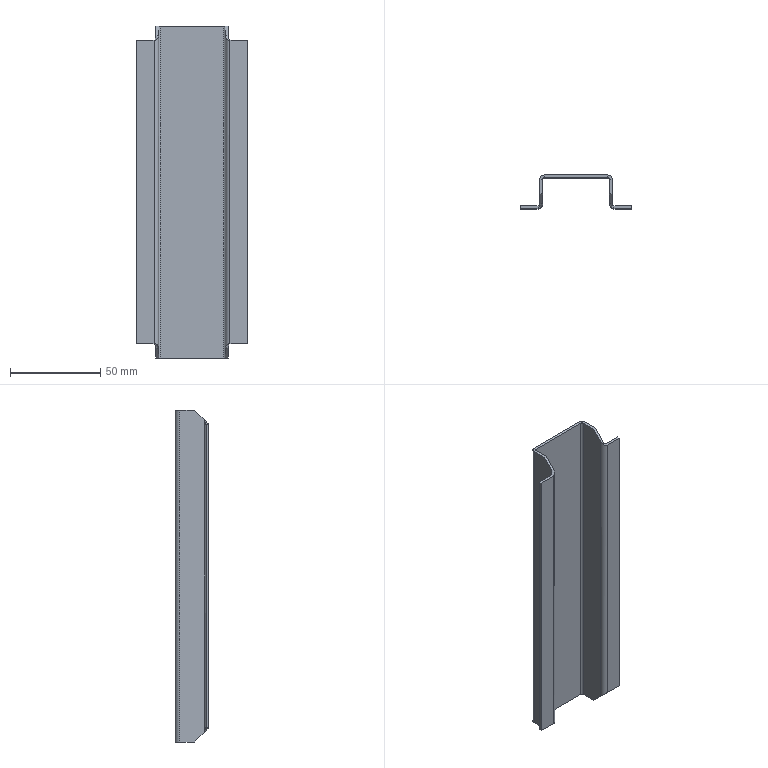Part | SolidWorks | features FlatPattern 1, ICE 1, SMBaseFlange 1, SheetMetal 1 | 1 solid | 42 faces | box 61 x 18.5 x 183.5 mm | volume 24658 mm3 | plane 30 | cylinder 8 | spline 4 | commonest cylinder face diameters 2 x4 5 x4
STEP:
#1=CARTESIAN_POINT('',(22.477,26.708,8.));
#2=VERTEX_POINT('',#1);
#3=CARTESIAN_POINT('',(12.977,26.708,8.));
#4=VERTEX_POINT('',#3);
#5=CARTESIAN_POINT('',(168.477,26.708,8.));
#6=DIRECTION('',(-1.,0.,0.));
#7=VECTOR('',#6,1000.);
#8=LINE('',#5,#7);
#9=EDGE_CURVE('',#2,#4,#8,.T.);
#10=ORIENTED_EDGE('',*,*,#9,.F.);
#11=CARTESIAN_POINT('',(22.477,26.708,175.5));
#12=VERTEX_POINT('',#11);
#13=CARTESIAN_POINT('',(22.477,26.708,183.5));
#14=DIRECTION('',(0.,0.,-1.));
#15=VECTOR('',#14,1000.);
#16=LINE('',#13,#15);
#17=EDGE_CURVE('',#12,#2,#16,.T.);
#18=ORIENTED_EDGE('',*,*,#17,.F.);
#19=CARTESIAN_POINT('',(12.977,26.708,175.5));
#20=VERTEX_POINT('',#19);
#21=CARTESIAN_POINT('',(168.477,26.708,175.5));
#22=DIRECTION('',(-1.,0.,0.));
#23=VECTOR('',#22,1000.);
#24=LINE('',#21,#23);
#25=EDGE_CURVE('',#12,#20,#24,.T.);
#26=ORIENTED_EDGE('',*,*,#25,.T.);
#27=CARTESIAN_POINT('',(12.977,26.708,183.5));
#28=DIRECTION('',(0.,0.,-1.));
#29=VECTOR('',#28,1000.);
#30=LINE('',#27,#29);
#31=EDGE_CURVE('',#20,#4,#30,.T.);
#32=ORIENTED_EDGE('',*,*,#31,.T.);
#33=EDGE_LOOP('',(#10,#18,#26,#32));
#34=FACE_OUTER_BOUND('',#33,.T.);
#35=CARTESIAN_POINT('',(11.977,26.708,183.5));
#36=DIRECTION('',(0.,1.,0.));
#37=DIRECTION('',(-1.,0.,0.));
#38=AXIS2_PLACEMENT_3D('',#35,#36,#37);
#39=PLANE('',#38);
#40=ADVANCED_FACE('',(#34),#39,.F.);
#41=ORIENTED_EDGE('',*,*,#17,.T.);
#42=CARTESIAN_POINT('',(22.477,28.208,8.));
#43=VERTEX_POINT('',#42);
#44=CARTESIAN_POINT('',(22.477,26.708,8.));
#45=DIRECTION('',(0.,1.,0.));
#46=VECTOR('',#45,1000.);
#47=LINE('',#44,#46);
#48=EDGE_CURVE('',#2,#43,#47,.T.);
#49=ORIENTED_EDGE('',*,*,#48,.T.);
#50=CARTESIAN_POINT('',(22.477,28.208,175.5));
#51=VERTEX_POINT('',#50);
#52=CARTESIAN_POINT('',(22.477,28.208,183.5));
#53=DIRECTION('',(0.,0.,-1.));
#54=VECTOR('',#53,1000.);
#55=LINE('',#52,#54);
#56=EDGE_CURVE('',#51,#43,#55,.T.);
#57=ORIENTED_EDGE('',*,*,#56,.F.);
#58=CARTESIAN_POINT('',(22.477,26.708,175.5));
#59=DIRECTION('',(0.,1.,0.));
#60=VECTOR('',#59,1000.);
#61=LINE('',#58,#60);
#62=EDGE_CURVE('',#12,#51,#61,.T.);
#63=ORIENTED_EDGE('',*,*,#62,.F.);
#64=EDGE_LOOP('',(#41,#49,#57,#63));
#65=FACE_OUTER_BOUND('',#64,.T.);
#66=CARTESIAN_POINT('',(22.477,28.208,183.5));
#67=DIRECTION('',(1.,0.,0.));
#68=DIRECTION('',(0.,0.,-1.));
#69=AXIS2_PLACEMENT_3D('',#66,#67,#68);
#70=PLANE('',#69);
#71=ADVANCED_FACE('',(#65),#70,.T.);
#72=ORIENTED_EDGE('',*,*,#56,.T.);
#73=CARTESIAN_POINT('',(12.977,28.208,8.));
#74=VERTEX_POINT('',#73);
#75=CARTESIAN_POINT('',(11.977,28.208,8.));
#76=DIRECTION('',(-1.,0.,0.));
#77=VECTOR('',#76,1000.);
#78=LINE('',#75,#77);
#79=EDGE_CURVE('',#43,#74,#78,.T.);
#80=ORIENTED_EDGE('',*,*,#79,.T.);
#81=CARTESIAN_POINT('',(12.977,28.208,175.5));
#82=VERTEX_POINT('',#81);
#83=CARTESIAN_POINT('',(12.977,28.208,183.5));
#84=DIRECTION('',(0.,0.,-1.));
#85=VECTOR('',#84,1000.);
#86=LINE('',#83,#85);
#87=EDGE_CURVE('',#82,#74,#86,.T.);
#88=ORIENTED_EDGE('',*,*,#87,.F.);
#89=CARTESIAN_POINT('',(11.977,28.208,175.5));
#90=DIRECTION('',(-1.,0.,0.));
#91=VECTOR('',#90,1000.);
#92=LINE('',#89,#91);
#93=EDGE_CURVE('',#51,#82,#92,.T.);
#94=ORIENTED_EDGE('',*,*,#93,.F.);
#95=EDGE_LOOP('',(#72,#80,#88,#94));
#96=FACE_OUTER_BOUND('',#95,.T.);
#97=CARTESIAN_POINT('',(11.977,28.208,183.5));
#98=DIRECTION('',(0.,1.,0.));
#99=DIRECTION('',(-1.,0.,0.));
#100=AXIS2_PLACEMENT_3D('',#97,#98,#99);
#101=PLANE('',#100);
#102=ADVANCED_FACE('',(#96),#101,.T.);
#103=ORIENTED_EDGE('',*,*,#87,.T.);
#104=CARTESIAN_POINT('',(11.977,29.208,5.5));
#105=VERTEX_POINT('',#104);
#106=CARTESIAN_POINT('',(11.977,29.208,5.5));
#107=CARTESIAN_POINT('',(11.977,28.623,6.964));
#108=CARTESIAN_POINT('',(12.391,28.208,8.));
#109=CARTESIAN_POINT('',(12.977,28.208,8.));
#110=(BOUNDED_CURVE()B_SPLINE_CURVE(3,(#106,#107,#108,#109),.UNSPECIFIED.,.F.,.T.)B_SPLINE_CURVE_WITH_KNOTS((4,4),(1.571,3.142),.UNSPECIFIED.)CURVE()GEOMETRIC_REPRESENTATION_ITEM()RATIONAL_B_SPLINE_CURVE((1.,0.8047,0.8047,1.))REPRESENTATION_ITEM(''));
#111=EDGE_CURVE('',#105,#74,#110,.T.);
#112=ORIENTED_EDGE('',*,*,#111,.F.);
#113=CARTESIAN_POINT('',(11.977,29.208,178.));
#114=VERTEX_POINT('',#113);
#115=CARTESIAN_POINT('',(11.977,29.208,183.5));
#116=DIRECTION('',(0.,0.,-1.));
#117=VECTOR('',#116,1000.);
#118=LINE('',#115,#117);
#119=EDGE_CURVE('',#114,#105,#118,.T.);
#120=ORIENTED_EDGE('',*,*,#119,.F.);
#121=CARTESIAN_POINT('',(12.977,28.208,175.5));
#122=CARTESIAN_POINT('',(12.391,28.208,175.5));
#123=CARTESIAN_POINT('',(11.977,28.623,176.536));
#124=CARTESIAN_POINT('',(11.977,29.208,178.));
#125=(BOUNDED_CURVE()B_SPLINE_CURVE(3,(#121,#122,#123,#124),.UNSPECIFIED.,.F.,.T.)B_SPLINE_CURVE_WITH_KNOTS((4,4),(0.,1.571),.UNSPECIFIED.)CURVE()GEOMETRIC_REPRESENTATION_ITEM()RATIONAL_B_SPLINE_CURVE((1.,0.8047,0.8047,1.))REPRESENTATION_ITEM(''));
#126=EDGE_CURVE('',#82,#114,#125,.T.);
#127=ORIENTED_EDGE('',*,*,#126,.F.);
#128=EDGE_LOOP('',(#103,#112,#120,#127));
#129=FACE_OUTER_BOUND('',#128,.T.);
#130=CARTESIAN_POINT('',(12.977,29.208,183.5));
#131=DIRECTION('',(0.,0.,-1.));
#132=DIRECTION('',(-1.,0.,0.));
#133=AXIS2_PLACEMENT_3D('',#130,#131,#132);
#134=CYLINDRICAL_SURFACE('',#133,1.);
#135=ADVANCED_FACE('',(#129),#134,.F.);
#136=ORIENTED_EDGE('',*,*,#119,.T.);
#137=CARTESIAN_POINT('',(11.977,34.708,0.));
#138=VERTEX_POINT('',#137);
#139=CARTESIAN_POINT('',(11.977,-51.792,86.5));
#140=DIRECTION('',(0.,-0.7071,0.7071));
#141=VECTOR('',#140,1000.);
#142=LINE('',#139,#141);
#143=EDGE_CURVE('',#138,#105,#142,.T.);
#144=ORIENTED_EDGE('',*,*,#143,.F.);
#145=CARTESIAN_POINT('',(11.977,42.708,0.));
#146=VERTEX_POINT('',#145);
#147=CARTESIAN_POINT('',(11.977,45.208,0.));
#148=DIRECTION('',(0.,-1.,0.));
#149=VECTOR('',#148,1000.);
#150=LINE('',#147,#149);
#151=EDGE_CURVE('',#146,#138,#150,.T.);
#152=ORIENTED_EDGE('',*,*,#151,.F.);
#153=CARTESIAN_POINT('',(11.977,42.708,183.5));
#154=VERTEX_POINT('',#153);
#155=CARTESIAN_POINT('',(11.977,42.708,183.5));
#156=DIRECTION('',(0.,0.,-1.));
#157=VECTOR('',#156,1000.);
#158=LINE('',#155,#157);
#159=EDGE_CURVE('',#154,#146,#158,.T.);
#160=ORIENTED_EDGE('',*,*,#159,.F.);
#161=CARTESIAN_POINT('',(11.977,34.708,183.5));
#162=VERTEX_POINT('',#161);
#163=CARTESIAN_POINT('',(11.977,45.208,183.5));
#164=DIRECTION('',(0.,-1.,0.));
#165=VECTOR('',#164,1000.);
#166=LINE('',#163,#165);
#167=EDGE_CURVE('',#154,#162,#166,.T.);
#168=ORIENTED_EDGE('',*,*,#167,.T.);
#169=CARTESIAN_POINT('',(11.977,39.958,188.75));
#170=DIRECTION('',(0.,0.7071,0.7071));
#171=VECTOR('',#170,1000.);
#172=LINE('',#169,#171);
#173=EDGE_CURVE('',#114,#162,#172,.T.);
#174=ORIENTED_EDGE('',*,*,#173,.F.);
#175=EDGE_LOOP('',(#136,#144,#152,#160,#168,#174));
#176=FACE_OUTER_BOUND('',#175,.T.);
#177=CARTESIAN_POINT('',(11.977,45.208,183.5));
#178=DIRECTION('',(1.,0.,0.));
#179=DIRECTION('',(0.,1.,0.));
#180=AXIS2_PLACEMENT_3D('',#177,#178,#179);
#181=PLANE('',#180);
#182=ADVANCED_FACE('',(#176),#181,.T.);
#183=CARTESIAN_POINT('',(10.477,34.708,0.));
#184=VERTEX_POINT('',#183);
#185=CARTESIAN_POINT('',(10.477,29.208,5.5));
#186=VERTEX_POINT('',#185);
#187=CARTESIAN_POINT('',(10.477,-51.792,86.5));
#188=DIRECTION('',(0.,-0.7071,0.7071));
#189=VECTOR('',#188,1000.);
#190=LINE('',#187,#189);
#191=EDGE_CURVE('',#184,#186,#190,.T.);
#192=ORIENTED_EDGE('',*,*,#191,.T.);
#193=CARTESIAN_POINT('',(10.477,29.208,178.));
#194=VERTEX_POINT('',#193);
#195=CARTESIAN_POINT('',(10.477,29.208,183.5));
#196=DIRECTION('',(0.,0.,-1.));
#197=VECTOR('',#196,1000.);
#198=LINE('',#195,#197);
#199=EDGE_CURVE('',#194,#186,#198,.T.);
#200=ORIENTED_EDGE('',*,*,#199,.F.);
#201=CARTESIAN_POINT('',(10.477,34.708,183.5));
#202=VERTEX_POINT('',#201);
#203=CARTESIAN_POINT('',(10.477,39.958,188.75));
#204=DIRECTION('',(0.,0.7071,0.7071));
#205=VECTOR('',#204,1000.);
#206=LINE('',#203,#205);
#207=EDGE_CURVE('',#194,#202,#206,.T.);
#208=ORIENTED_EDGE('',*,*,#207,.T.);
#209=CARTESIAN_POINT('',(10.477,42.708,183.5));
#210=VERTEX_POINT('',#209);
#211=CARTESIAN_POINT('',(10.477,45.208,183.5));
#212=DIRECTION('',(0.,-1.,0.));
#213=VECTOR('',#212,1000.);
#214=LINE('',#211,#213);
#215=EDGE_CURVE('',#210,#202,#214,.T.);
#216=ORIENTED_EDGE('',*,*,#215,.F.);
#217=CARTESIAN_POINT('',(10.477,42.708,0.));
#218=VERTEX_POINT('',#217);
#219=CARTESIAN_POINT('',(10.477,42.708,183.5));
#220=DIRECTION('',(0.,0.,-1.));
#221=VECTOR('',#220,1000.);
#222=LINE('',#219,#221);
#223=EDGE_CURVE('',#210,#218,#222,.T.);
#224=ORIENTED_EDGE('',*,*,#223,.T.);
#225=CARTESIAN_POINT('',(10.477,45.208,0.));
#226=DIRECTION('',(0.,-1.,0.));
#227=VECTOR('',#226,1000.);
#228=LINE('',#225,#227);
#229=EDGE_CURVE('',#218,#184,#228,.T.);
#230=ORIENTED_EDGE('',*,*,#229,.T.);
#231=EDGE_LOOP('',(#192,#200,#208,#216,#224,#230));
#232=FACE_OUTER_BOUND('',#231,.T.);
#233=CARTESIAN_POINT('',(10.477,45.208,183.5));
#234=DIRECTION('',(1.,0.,0.));
#235=DIRECTION('',(0.,1.,0.));
#236=AXIS2_PLACEMENT_3D('',#233,#234,#235);
#237=PLANE('',#236);
#238=ADVANCED_FACE('',(#232),#237,.F.);
#239=CARTESIAN_POINT('',(10.477,29.208,5.5));
#240=CARTESIAN_POINT('',(10.477,27.744,6.964));
#241=CARTESIAN_POINT('',(11.512,26.708,8.));
#242=CARTESIAN_POINT('',(12.977,26.708,8.));
#243=(BOUNDED_CURVE()B_SPLINE_CURVE(3,(#239,#240,#241,#242),.UNSPECIFIED.,.F.,.T.)B_SPLINE_CURVE_WITH_KNOTS((4,4),(1.571,3.142),.UNSPECIFIED.)CURVE()GEOMETRIC_REPRESENTATION_ITEM()RATIONAL_B_SPLINE_CURVE((1.,0.8047,0.8047,1.))REPRESENTATION_ITEM(''));
#244=EDGE_CURVE('',#186,#4,#243,.T.);
#245=ORIENTED_EDGE('',*,*,#244,.T.);
#246=ORIENTED_EDGE('',*,*,#31,.F.);
#247=CARTESIAN_POINT('',(12.977,26.708,175.5));
#248=CARTESIAN_POINT('',(11.512,26.708,175.5));
#249=CARTESIAN_POINT('',(10.477,27.744,176.536));
#250=CARTESIAN_POINT('',(10.477,29.208,178.));
#251=(BOUNDED_CURVE()B_SPLINE_CURVE(3,(#247,#248,#249,#250),.UNSPECIFIED.,.F.,.T.)B_SPLINE_CURVE_WITH_KNOTS((4,4),(0.,1.571),.UNSPECIFIED.)CURVE()GEOMETRIC_REPRESENTATION_ITEM()RATIONAL_B_SPLINE_CURVE((1.,0.8047,0.8047,1.))REPRESENTATION_ITEM(''));
#252=EDGE_CURVE('',#20,#194,#251,.T.);
#253=ORIENTED_EDGE('',*,*,#252,.T.);
#254=ORIENTED_EDGE('',*,*,#199,.T.);
#255=EDGE_LOOP('',(#245,#246,#253,#254));
#256=FACE_OUTER_BOUND('',#255,.T.);
#257=CARTESIAN_POINT('',(12.977,29.208,183.5));
#258=DIRECTION('',(0.,0.,-1.));
#259=DIRECTION('',(-1.,0.,0.));
#260=AXIS2_PLACEMENT_3D('',#257,#258,#259);
#261=CYLINDRICAL_SURFACE('',#260,2.5);
#262=ADVANCED_FACE('',(#256),#261,.T.);
#263=CARTESIAN_POINT('',(-28.023,34.708,0.));
#264=VERTEX_POINT('',#263);
#265=CARTESIAN_POINT('',(-28.023,42.708,0.));
#266=VERTEX_POINT('',#265);
#267=CARTESIAN_POINT('',(-28.023,28.208,0.));
#268=DIRECTION('',(0.,1.,0.));
#269=VECTOR('',#268,1000.);
#270=LINE('',#267,#269);
#271=EDGE_CURVE('',#264,#266,#270,.T.);
#272=ORIENTED_EDGE('',*,*,#271,.F.);
#273=CARTESIAN_POINT('',(-28.023,29.208,5.5));
#274=VERTEX_POINT('',#273);
#275=CARTESIAN_POINT('',(-28.023,-60.292,95.));
#276=DIRECTION('',(0.,0.7071,-0.7071));
#277=VECTOR('',#276,1000.);
#278=LINE('',#275,#277);
#279=EDGE_CURVE('',#274,#264,#278,.T.);
#280=ORIENTED_EDGE('',*,*,#279,.F.);
#281=CARTESIAN_POINT('',(-28.023,29.208,178.));
#282=VERTEX_POINT('',#281);
#283=CARTESIAN_POINT('',(-28.023,29.208,183.5));
#284=DIRECTION('',(0.,0.,-1.));
#285=VECTOR('',#284,1000.);
#286=LINE('',#283,#285);
#287=EDGE_CURVE('',#282,#274,#286,.T.);
#288=ORIENTED_EDGE('',*,*,#287,.F.);
#289=CARTESIAN_POINT('',(-28.023,34.708,183.5));
#290=VERTEX_POINT('',#289);
#291=CARTESIAN_POINT('',(-28.023,31.458,180.25));
#292=DIRECTION('',(0.,-0.7071,-0.7071));
#293=VECTOR('',#292,1000.);
#294=LINE('',#291,#293);
#295=EDGE_CURVE('',#290,#282,#294,.T.);
#296=ORIENTED_EDGE('',*,*,#295,.F.);
#297=CARTESIAN_POINT('',(-28.023,42.708,183.5));
#298=VERTEX_POINT('',#297);
#299=CARTESIAN_POINT('',(-28.023,28.208,183.5));
#300=DIRECTION('',(0.,1.,0.));
#301=VECTOR('',#300,1000.);
#302=LINE('',#299,#301);
#303=EDGE_CURVE('',#290,#298,#302,.T.);
#304=ORIENTED_EDGE('',*,*,#303,.T.);
#305=CARTESIAN_POINT('',(-28.023,42.708,183.5));
#306=DIRECTION('',(0.,0.,-1.));
#307=VECTOR('',#306,1000.);
#308=LINE('',#305,#307);
#309=EDGE_CURVE('',#298,#266,#308,.T.);
#310=ORIENTED_EDGE('',*,*,#309,.T.);
#311=EDGE_LOOP('',(#272,#280,#288,#296,#304,#310));
#312=FACE_OUTER_BOUND('',#311,.T.);
#313=CARTESIAN_POINT('',(-28.023,28.208,183.5));
#314=DIRECTION('',(-1.,0.,0.));
#315=DIRECTION('',(0.,0.,1.));
#316=AXIS2_PLACEMENT_3D('',#313,#314,#315);
#317=PLANE('',#316);
#318=ADVANCED_FACE('',(#312),#317,.T.);
#319=ORIENTED_EDGE('',*,*,#287,.T.);
#320=CARTESIAN_POINT('',(-29.023,28.208,8.));
#321=VERTEX_POINT('',#320);
#322=CARTESIAN_POINT('',(-29.023,28.208,8.));
#323=CARTESIAN_POINT('',(-28.437,28.208,8.));
#324=CARTESIAN_POINT('',(-28.023,28.623,6.964));
#325=CARTESIAN_POINT('',(-28.023,29.208,5.5));
#326=(BOUNDED_CURVE()B_SPLINE_CURVE(3,(#322,#323,#324,#325),.UNSPECIFIED.,.F.,.T.)B_SPLINE_CURVE_WITH_KNOTS((4,4),(3.142,4.712),.UNSPECIFIED.)CURVE()GEOMETRIC_REPRESENTATION_ITEM()RATIONAL_B_SPLINE_CURVE((1.,0.8047,0.8047,1.))REPRESENTATION_ITEM(''));
#327=EDGE_CURVE('',#321,#274,#326,.T.);
#328=ORIENTED_EDGE('',*,*,#327,.F.);
#329=CARTESIAN_POINT('',(-29.023,28.208,175.5));
#330=VERTEX_POINT('',#329);
#331=CARTESIAN_POINT('',(-29.023,28.208,183.5));
#332=DIRECTION('',(0.,0.,-1.));
#333=VECTOR('',#332,1000.);
#334=LINE('',#331,#333);
#335=EDGE_CURVE('',#330,#321,#334,.T.);
#336=ORIENTED_EDGE('',*,*,#335,.F.);
#337=CARTESIAN_POINT('',(-28.023,29.208,178.));
#338=CARTESIAN_POINT('',(-28.023,28.623,176.536));
#339=CARTESIAN_POINT('',(-28.437,28.208,175.5));
#340=CARTESIAN_POINT('',(-29.023,28.208,175.5));
#341=(BOUNDED_CURVE()B_SPLINE_CURVE(3,(#337,#338,#339,#340),.UNSPECIFIED.,.F.,.T.)B_SPLINE_CURVE_WITH_KNOTS((4,4),(4.712,6.283),.UNSPECIFIED.)CURVE()GEOMETRIC_REPRESENTATION_ITEM()RATIONAL_B_SPLINE_CURVE((1.,0.8047,0.8047,1.))REPRESENTATION_ITEM(''));
#342=EDGE_CURVE('',#282,#330,#341,.T.);
#343=ORIENTED_EDGE('',*,*,#342,.F.);
#344=EDGE_LOOP('',(#319,#328,#336,#343));
#345=FACE_OUTER_BOUND('',#344,.T.);
#346=CARTESIAN_POINT('',(-29.023,29.208,183.5));
#347=DIRECTION('',(0.,0.,-1.));
#348=DIRECTION('',(-1.,0.,0.));
#349=AXIS2_PLACEMENT_3D('',#346,#347,#348);
#350=CYLINDRICAL_SURFACE('',#349,1.);
#351=ADVANCED_FACE('',(#345),#350,.F.);
#352=ORIENTED_EDGE('',*,*,#335,.T.);
#353=CARTESIAN_POINT('',(-38.523,28.208,8.));
#354=VERTEX_POINT('',#353);
#355=CARTESIAN_POINT('',(-38.523,28.208,8.));
#356=DIRECTION('',(-1.,0.,0.));
#357=VECTOR('',#356,1000.);
#358=LINE('',#355,#357);
#359=EDGE_CURVE('',#321,#354,#358,.T.);
#360=ORIENTED_EDGE('',*,*,#359,.T.);
#361=CARTESIAN_POINT('',(-38.523,28.208,175.5));
#362=VERTEX_POINT('',#361);
#363=CARTESIAN_POINT('',(-38.523,28.208,183.5));
#364=DIRECTION('',(0.,0.,-1.));
#365=VECTOR('',#364,1000.);
#366=LINE('',#363,#365);
#367=EDGE_CURVE('',#362,#354,#366,.T.);
#368=ORIENTED_EDGE('',*,*,#367,.F.);
#369=CARTESIAN_POINT('',(-38.523,28.208,175.5));
#370=DIRECTION('',(-1.,0.,0.));
#371=VECTOR('',#370,1000.);
#372=LINE('',#369,#371);
#373=EDGE_CURVE('',#330,#362,#372,.T.);
#374=ORIENTED_EDGE('',*,*,#373,.F.);
#375=EDGE_LOOP('',(#352,#360,#368,#374));
#376=FACE_OUTER_BOUND('',#375,.T.);
#377=CARTESIAN_POINT('',(-38.523,28.208,183.5));
#378=DIRECTION('',(0.,1.,0.));
#379=DIRECTION('',(0.,0.,1.));
#380=AXIS2_PLACEMENT_3D('',#377,#378,#379);
#381=PLANE('',#380);
#382=ADVANCED_FACE('',(#376),#381,.T.);
#383=ORIENTED_EDGE('',*,*,#367,.T.);
#384=CARTESIAN_POINT('',(-38.523,26.708,8.));
#385=VERTEX_POINT('',#384);
#386=CARTESIAN_POINT('',(-38.523,26.708,8.));
#387=DIRECTION('',(0.,1.,0.));
#388=VECTOR('',#387,1000.);
#389=LINE('',#386,#388);
#390=EDGE_CURVE('',#385,#354,#389,.T.);
#391=ORIENTED_EDGE('',*,*,#390,.F.);
#392=CARTESIAN_POINT('',(-38.523,26.708,175.5));
#393=VERTEX_POINT('',#392);
#394=CARTESIAN_POINT('',(-38.523,26.708,183.5));
#395=DIRECTION('',(0.,0.,-1.));
#396=VECTOR('',#395,1000.);
#397=LINE('',#394,#396);
#398=EDGE_CURVE('',#393,#385,#397,.T.);
#399=ORIENTED_EDGE('',*,*,#398,.F.);
#400=CARTESIAN_POINT('',(-38.523,26.708,175.5));
#401=DIRECTION('',(0.,1.,0.));
#402=VECTOR('',#401,1000.);
#403=LINE('',#400,#402);
#404=EDGE_CURVE('',#393,#362,#403,.T.);
#405=ORIENTED_EDGE('',*,*,#404,.T.);
#406=EDGE_LOOP('',(#383,#391,#399,#405));
#407=FACE_OUTER_BOUND('',#406,.T.);
#408=CARTESIAN_POINT('',(-38.523,26.708,183.5));
#409=DIRECTION('',(-1.,0.,0.));
#410=DIRECTION('',(0.,0.,1.));
#411=AXIS2_PLACEMENT_3D('',#408,#409,#410);
#412=PLANE('',#411);
#413=ADVANCED_FACE('',(#407),#412,.T.);
#414=CARTESIAN_POINT('',(-29.023,26.708,8.));
#415=VERTEX_POINT('',#414);
#416=CARTESIAN_POINT('',(168.477,26.708,8.));
#417=DIRECTION('',(-1.,0.,0.));
#418=VECTOR('',#417,1000.);
#419=LINE('',#416,#418);
#420=EDGE_CURVE('',#415,#385,#419,.T.);
#421=ORIENTED_EDGE('',*,*,#420,.F.);
#422=CARTESIAN_POINT('',(-29.023,26.708,175.5));
#423=VERTEX_POINT('',#422);
#424=CARTESIAN_POINT('',(-29.023,26.708,183.5));
#425=DIRECTION('',(0.,0.,-1.));
#426=VECTOR('',#425,1000.);
#427=LINE('',#424,#426);
#428=EDGE_CURVE('',#423,#415,#427,.T.);
#429=ORIENTED_EDGE('',*,*,#428,.F.);
#430=CARTESIAN_POINT('',(168.477,26.708,175.5));
#431=DIRECTION('',(-1.,0.,0.));
#432=VECTOR('',#431,1000.);
#433=LINE('',#430,#432);
#434=EDGE_CURVE('',#423,#393,#433,.T.);
#435=ORIENTED_EDGE('',*,*,#434,.T.);
#436=ORIENTED_EDGE('',*,*,#398,.T.);
#437=EDGE_LOOP('',(#421,#429,#435,#436));
#438=FACE_OUTER_BOUND('',#437,.T.);
#439=CARTESIAN_POINT('',(-38.523,26.708,183.5));
#440=DIRECTION('',(0.,1.,0.));
#441=DIRECTION('',(0.,0.,1.));
#442=AXIS2_PLACEMENT_3D('',#439,#440,#441);
#443=PLANE('',#442);
#444=ADVANCED_FACE('',(#438),#443,.F.);
#445=CARTESIAN_POINT('',(-26.523,29.208,5.5));
#446=VERTEX_POINT('',#445);
#447=CARTESIAN_POINT('',(-29.023,26.708,8.));
#448=CARTESIAN_POINT('',(-27.559,26.708,8.));
#449=CARTESIAN_POINT('',(-26.523,27.744,6.964));
#450=CARTESIAN_POINT('',(-26.523,29.208,5.5));
#451=(BOUNDED_CURVE()B_SPLINE_CURVE(3,(#447,#448,#449,#450),.UNSPECIFIED.,.F.,.T.)B_SPLINE_CURVE_WITH_KNOTS((4,4),(3.142,4.712),.UNSPECIFIED.)CURVE()GEOMETRIC_REPRESENTATION_ITEM()RATIONAL_B_SPLINE_CURVE((1.,0.8047,0.8047,1.))REPRESENTATION_ITEM(''));
#452=EDGE_CURVE('',#415,#446,#451,.T.);
#453=ORIENTED_EDGE('',*,*,#452,.T.);
#454=CARTESIAN_POINT('',(-26.523,29.208,178.));
#455=VERTEX_POINT('',#454);
#456=CARTESIAN_POINT('',(-26.523,29.208,183.5));
#457=DIRECTION('',(0.,0.,-1.));
#458=VECTOR('',#457,1000.);
#459=LINE('',#456,#458);
#460=EDGE_CURVE('',#455,#446,#459,.T.);
#461=ORIENTED_EDGE('',*,*,#460,.F.);
#462=CARTESIAN_POINT('',(-26.523,29.208,178.));
#463=CARTESIAN_POINT('',(-26.523,27.744,176.536));
#464=CARTESIAN_POINT('',(-27.559,26.708,175.5));
#465=CARTESIAN_POINT('',(-29.023,26.708,175.5));
#466=(BOUNDED_CURVE()B_SPLINE_CURVE(3,(#462,#463,#464,#465),.UNSPECIFIED.,.F.,.T.)B_SPLINE_CURVE_WITH_KNOTS((4,4),(4.712,6.283),.UNSPECIFIED.)CURVE()GEOMETRIC_REPRESENTATION_ITEM()RATIONAL_B_SPLINE_CURVE((1.,0.8047,0.8047,1.))REPRESENTATION_ITEM(''));
#467=EDGE_CURVE('',#455,#423,#466,.T.);
#468=ORIENTED_EDGE('',*,*,#467,.T.);
#469=ORIENTED_EDGE('',*,*,#428,.T.);
#470=EDGE_LOOP('',(#453,#461,#468,#469));
#471=FACE_OUTER_BOUND('',#470,.T.);
#472=CARTESIAN_POINT('',(-29.023,29.208,183.5));
#473=DIRECTION('',(0.,0.,-1.));
#474=DIRECTION('',(-1.,0.,0.));
#475=AXIS2_PLACEMENT_3D('',#472,#473,#474);
#476=CYLINDRICAL_SURFACE('',#475,2.5);
#477=ADVANCED_FACE('',(#471),#476,.T.);
#478=CARTESIAN_POINT('',(-26.523,34.708,0.));
#479=VERTEX_POINT('',#478);
#480=CARTESIAN_POINT('',(-26.523,-60.292,95.));
#481=DIRECTION('',(0.,0.7071,-0.7071));
#482=VECTOR('',#481,1000.);
#483=LINE('',#480,#482);
#484=EDGE_CURVE('',#446,#479,#483,.T.);
#485=ORIENTED_EDGE('',*,*,#484,.T.);
#486=CARTESIAN_POINT('',(-26.523,42.708,0.));
#487=VERTEX_POINT('',#486);
#488=CARTESIAN_POINT('',(-26.523,28.208,0.));
#489=DIRECTION('',(0.,1.,0.));
#490=VECTOR('',#489,1000.);
#491=LINE('',#488,#490);
#492=EDGE_CURVE('',#479,#487,#491,.T.);
#493=ORIENTED_EDGE('',*,*,#492,.T.);
#494=CARTESIAN_POINT('',(-26.523,42.708,183.5));
#495=VERTEX_POINT('',#494);
#496=CARTESIAN_POINT('',(-26.523,42.708,183.5));
#497=DIRECTION('',(0.,0.,-1.));
#498=VECTOR('',#497,1000.);
#499=LINE('',#496,#498);
#500=EDGE_CURVE('',#495,#487,#499,.T.);
#501=ORIENTED_EDGE('',*,*,#500,.F.);
#502=CARTESIAN_POINT('',(-26.523,34.708,183.5));
#503=VERTEX_POINT('',#502);
#504=CARTESIAN_POINT('',(-26.523,28.208,183.5));
#505=DIRECTION('',(0.,1.,0.));
#506=VECTOR('',#505,1000.);
#507=LINE('',#504,#506);
#508=EDGE_CURVE('',#503,#495,#507,.T.);
#509=ORIENTED_EDGE('',*,*,#508,.F.);
#510=CARTESIAN_POINT('',(-26.523,31.458,180.25));
#511=DIRECTION('',(0.,-0.7071,-0.7071));
#512=VECTOR('',#511,1000.);
#513=LINE('',#510,#512);
#514=EDGE_CURVE('',#503,#455,#513,.T.);
#515=ORIENTED_EDGE('',*,*,#514,.T.);
#516=ORIENTED_EDGE('',*,*,#460,.T.);
#517=EDGE_LOOP('',(#485,#493,#501,#509,#515,#516));
#518=FACE_OUTER_BOUND('',#517,.T.);
#519=CARTESIAN_POINT('',(-26.523,28.208,183.5));
#520=DIRECTION('',(-1.,0.,0.));
#521=DIRECTION('',(0.,0.,1.));
#522=AXIS2_PLACEMENT_3D('',#519,#520,#521);
#523=PLANE('',#522);
#524=ADVANCED_FACE('',(#518),#523,.F.);
#525=ORIENTED_EDGE('',*,*,#303,.F.);
#526=CARTESIAN_POINT('',(-28.023,34.708,183.5));
#527=DIRECTION('',(1.,0.,0.));
#528=VECTOR('',#527,1000.);
#529=LINE('',#526,#528);
#530=EDGE_CURVE('',#290,#503,#529,.T.);
#531=ORIENTED_EDGE('',*,*,#530,.T.);
#532=ORIENTED_EDGE('',*,*,#508,.T.);
#533=CARTESIAN_POINT('',(-26.523,42.708,183.5));
#534=DIRECTION('',(-1.,0.,0.));
#535=VECTOR('',#534,1000.);
#536=LINE('',#533,#535);
#537=EDGE_CURVE('',#495,#298,#536,.T.);
#538=ORIENTED_EDGE('',*,*,#537,.T.);
#539=EDGE_LOOP('',(#525,#531,#532,#538));
#540=FACE_OUTER_BOUND('',#539,.T.);
#541=CARTESIAN_POINT('',(-29.023,26.708,183.5));
#542=DIRECTION('',(0.,0.,1.));
#543=DIRECTION('',(1.,0.,0.));
#544=AXIS2_PLACEMENT_3D('',#541,#542,#543);
#545=PLANE('',#544);
#546=ADVANCED_FACE('',(#540),#545,.T.);
#547=CARTESIAN_POINT('',(-25.523,45.208,183.5));
#548=VERTEX_POINT('',#547);
#549=CARTESIAN_POINT('',(-25.523,43.708,183.5));
#550=VERTEX_POINT('',#549);
#551=CARTESIAN_POINT('',(-25.523,45.208,183.5));
#552=DIRECTION('',(0.,-1.,0.));
#553=VECTOR('',#552,1000.);
#554=LINE('',#551,#553);
#555=EDGE_CURVE('',#548,#550,#554,.T.);
#556=ORIENTED_EDGE('',*,*,#555,.F.);
#557=CARTESIAN_POINT('',(-25.523,42.708,183.5));
#558=DIRECTION('',(0.,0.,-1.));
#559=DIRECTION('',(1.,0.,0.));
#560=AXIS2_PLACEMENT_3D('',#557,#558,#559);
#561=CIRCLE('',#560,2.5);
#562=EDGE_CURVE('',#298,#548,#561,.T.);
#563=ORIENTED_EDGE('',*,*,#562,.F.);
#564=ORIENTED_EDGE('',*,*,#537,.F.);
#565=CARTESIAN_POINT('',(-25.523,42.708,183.5));
#566=DIRECTION('',(0.,0.,-1.));
#567=DIRECTION('',(1.,0.,0.));
#568=AXIS2_PLACEMENT_3D('',#565,#566,#567);
#569=CIRCLE('',#568,1.);
#570=EDGE_CURVE('',#495,#550,#569,.T.);
#571=ORIENTED_EDGE('',*,*,#570,.T.);
#572=EDGE_LOOP('',(#556,#563,#564,#571));
#573=FACE_OUTER_BOUND('',#572,.T.);
#574=CARTESIAN_POINT('',(-25.523,45.208,183.5));
#575=DIRECTION('',(0.,0.,1.));
#576=DIRECTION('',(1.,0.,0.));
#577=AXIS2_PLACEMENT_3D('',#574,#575,#576);
#578=PLANE('',#577);
#579=ADVANCED_FACE('',(#573),#578,.T.);
#580=CARTESIAN_POINT('',(9.477,45.208,183.5));
#581=VERTEX_POINT('',#580);
#582=CARTESIAN_POINT('',(-28.023,45.208,183.5));
#583=DIRECTION('',(1.,0.,0.));
#584=VECTOR('',#583,1000.);
#585=LINE('',#582,#584);
#586=EDGE_CURVE('',#548,#581,#585,.T.);
#587=ORIENTED_EDGE('',*,*,#586,.F.);
#588=ORIENTED_EDGE('',*,*,#555,.T.);
#589=CARTESIAN_POINT('',(9.477,43.708,183.5));
#590=VERTEX_POINT('',#589);
#591=CARTESIAN_POINT('',(-28.023,43.708,183.5));
#592=DIRECTION('',(1.,0.,0.));
#593=VECTOR('',#592,1000.);
#594=LINE('',#591,#593);
#595=EDGE_CURVE('',#550,#590,#594,.T.);
#596=ORIENTED_EDGE('',*,*,#595,.T.);
#597=CARTESIAN_POINT('',(9.477,43.708,183.5));
#598=DIRECTION('',(0.,1.,0.));
#599=VECTOR('',#598,1000.);
#600=LINE('',#597,#599);
#601=EDGE_CURVE('',#590,#581,#600,.T.);
#602=ORIENTED_EDGE('',*,*,#601,.T.);
#603=EDGE_LOOP('',(#587,#588,#596,#602));
#604=FACE_OUTER_BOUND('',#603,.T.);
#605=CARTESIAN_POINT('',(-26.523,42.708,183.5));
#606=DIRECTION('',(0.,0.,1.));
#607=DIRECTION('',(1.,0.,0.));
#608=AXIS2_PLACEMENT_3D('',#605,#606,#607);
#609=PLANE('',#608);
#610=ADVANCED_FACE('',(#604),#609,.T.);
#611=CARTESIAN_POINT('',(-28.023,42.708,0.));
#612=DIRECTION('',(1.,0.,0.));
#613=VECTOR('',#612,1000.);
#614=LINE('',#611,#613);
#615=EDGE_CURVE('',#266,#487,#614,.T.);
#616=ORIENTED_EDGE('',*,*,#615,.F.);
#617=CARTESIAN_POINT('',(-25.523,45.208,0.));
#618=VERTEX_POINT('',#617);
#619=CARTESIAN_POINT('',(-25.523,42.708,0.));
#620=DIRECTION('',(0.,0.,-1.));
#621=DIRECTION('',(1.,0.,0.));
#622=AXIS2_PLACEMENT_3D('',#619,#620,#621);
#623=CIRCLE('',#622,2.5);
#624=EDGE_CURVE('',#266,#618,#623,.T.);
#625=ORIENTED_EDGE('',*,*,#624,.T.);
#626=CARTESIAN_POINT('',(-25.523,43.708,0.));
#627=VERTEX_POINT('',#626);
#628=CARTESIAN_POINT('',(-25.523,43.708,0.));
#629=DIRECTION('',(0.,1.,0.));
#630=VECTOR('',#629,1000.);
#631=LINE('',#628,#630);
#632=EDGE_CURVE('',#627,#618,#631,.T.);
#633=ORIENTED_EDGE('',*,*,#632,.F.);
#634=CARTESIAN_POINT('',(-25.523,42.708,0.));
#635=DIRECTION('',(0.,0.,-1.));
#636=DIRECTION('',(1.,0.,0.));
#637=AXIS2_PLACEMENT_3D('',#634,#635,#636);
#638=CIRCLE('',#637,1.);
#639=EDGE_CURVE('',#487,#627,#638,.T.);
#640=ORIENTED_EDGE('',*,*,#639,.F.);
#641=EDGE_LOOP('',(#616,#625,#633,#640));
#642=FACE_OUTER_BOUND('',#641,.T.);
#643=CARTESIAN_POINT('',(-28.023,42.708,0.));
#644=DIRECTION('',(0.,0.,-1.));
#645=DIRECTION('',(-1.,0.,0.));
#646=AXIS2_PLACEMENT_3D('',#643,#644,#645);
#647=PLANE('',#646);
#648=ADVANCED_FACE('',(#642),#647,.T.);
#649=ORIENTED_EDGE('',*,*,#492,.F.);
#650=CARTESIAN_POINT('',(-28.023,34.708,0.));
#651=DIRECTION('',(1.,0.,0.));
#652=VECTOR('',#651,1000.);
#653=LINE('',#650,#652);
#654=EDGE_CURVE('',#264,#479,#653,.T.);
#655=ORIENTED_EDGE('',*,*,#654,.F.);
#656=ORIENTED_EDGE('',*,*,#271,.T.);
#657=ORIENTED_EDGE('',*,*,#615,.T.);
#658=EDGE_LOOP('',(#649,#655,#656,#657));
#659=FACE_OUTER_BOUND('',#658,.T.);
#660=CARTESIAN_POINT('',(-25.523,43.708,0.));
#661=DIRECTION('',(0.,0.,-1.));
#662=DIRECTION('',(-1.,0.,0.));
#663=AXIS2_PLACEMENT_3D('',#660,#661,#662);
#664=PLANE('',#663);
#665=ADVANCED_FACE('',(#659),#664,.T.);
#666=CARTESIAN_POINT('',(11.977,42.708,183.5));
#667=DIRECTION('',(-1.,0.,0.));
#668=VECTOR('',#667,1000.);
#669=LINE('',#666,#668);
#670=EDGE_CURVE('',#154,#210,#669,.T.);
#671=ORIENTED_EDGE('',*,*,#670,.F.);
#672=CARTESIAN_POINT('',(9.477,42.708,183.5));
#673=DIRECTION('',(0.,0.,-1.));
#674=DIRECTION('',(1.,0.,0.));
#675=AXIS2_PLACEMENT_3D('',#672,#673,#674);
#676=CIRCLE('',#675,2.5);
#677=EDGE_CURVE('',#581,#154,#676,.T.);
#678=ORIENTED_EDGE('',*,*,#677,.F.);
#679=ORIENTED_EDGE('',*,*,#601,.F.);
#680=CARTESIAN_POINT('',(9.477,42.708,183.5));
#681=DIRECTION('',(0.,0.,-1.));
#682=DIRECTION('',(1.,0.,0.));
#683=AXIS2_PLACEMENT_3D('',#680,#681,#682);
#684=CIRCLE('',#683,1.);
#685=EDGE_CURVE('',#590,#210,#684,.T.);
#686=ORIENTED_EDGE('',*,*,#685,.T.);
#687=EDGE_LOOP('',(#671,#678,#679,#686));
#688=FACE_OUTER_BOUND('',#687,.T.);
#689=CARTESIAN_POINT('',(11.977,42.708,183.5));
#690=DIRECTION('',(0.,0.,1.));
#691=DIRECTION('',(1.,0.,0.));
#692=AXIS2_PLACEMENT_3D('',#689,#690,#691);
#693=PLANE('',#692);
#694=ADVANCED_FACE('',(#688),#693,.T.);
#695=ORIENTED_EDGE('',*,*,#215,.T.);
#696=CARTESIAN_POINT('',(10.477,34.708,183.5));
#697=DIRECTION('',(1.,0.,0.));
#698=VECTOR('',#697,1000.);
#699=LINE('',#696,#698);
#700=EDGE_CURVE('',#202,#162,#699,.T.);
#701=ORIENTED_EDGE('',*,*,#700,.T.);
#702=ORIENTED_EDGE('',*,*,#167,.F.);
#703=ORIENTED_EDGE('',*,*,#670,.T.);
#704=EDGE_LOOP('',(#695,#701,#702,#703));
#705=FACE_OUTER_BOUND('',#704,.T.);
#706=CARTESIAN_POINT('',(9.477,43.708,183.5));
#707=DIRECTION('',(0.,0.,1.));
#708=DIRECTION('',(1.,0.,0.));
#709=AXIS2_PLACEMENT_3D('',#706,#707,#708);
#710=PLANE('',#709);
#711=ADVANCED_FACE('',(#705),#710,.T.);
#712=CARTESIAN_POINT('',(9.477,45.208,0.));
#713=VERTEX_POINT('',#712);
#714=CARTESIAN_POINT('',(9.477,43.708,0.));
#715=VERTEX_POINT('',#714);
#716=CARTESIAN_POINT('',(9.477,45.208,0.));
#717=DIRECTION('',(0.,-1.,0.));
#718=VECTOR('',#717,1000.);
#719=LINE('',#716,#718);
#720=EDGE_CURVE('',#713,#715,#719,.T.);
#721=ORIENTED_EDGE('',*,*,#720,.F.);
#722=CARTESIAN_POINT('',(9.477,42.708,0.));
#723=DIRECTION('',(0.,0.,-1.));
#724=DIRECTION('',(1.,0.,0.));
#725=AXIS2_PLACEMENT_3D('',#722,#723,#724);
#726=CIRCLE('',#725,2.5);
#727=EDGE_CURVE('',#713,#146,#726,.T.);
#728=ORIENTED_EDGE('',*,*,#727,.T.);
#729=CARTESIAN_POINT('',(10.477,42.708,0.));
#730=DIRECTION('',(1.,0.,0.));
#731=VECTOR('',#730,1000.);
#732=LINE('',#729,#731);
#733=EDGE_CURVE('',#218,#146,#732,.T.);
#734=ORIENTED_EDGE('',*,*,#733,.F.);
#735=CARTESIAN_POINT('',(9.477,42.708,0.));
#736=DIRECTION('',(0.,0.,-1.));
#737=DIRECTION('',(1.,0.,0.));
#738=AXIS2_PLACEMENT_3D('',#735,#736,#737);
#739=CIRCLE('',#738,1.);
#740=EDGE_CURVE('',#715,#218,#739,.T.);
#741=ORIENTED_EDGE('',*,*,#740,.F.);
#742=EDGE_LOOP('',(#721,#728,#734,#741));
#743=FACE_OUTER_BOUND('',#742,.T.);
#744=CARTESIAN_POINT('',(9.477,45.208,0.));
#745=DIRECTION('',(0.,0.,-1.));
#746=DIRECTION('',(-1.,0.,0.));
#747=AXIS2_PLACEMENT_3D('',#744,#745,#746);
#748=PLANE('',#747);
#749=ADVANCED_FACE('',(#743),#748,.T.);
#750=CARTESIAN_POINT('',(-28.023,45.208,0.));
#751=DIRECTION('',(1.,0.,0.));
#752=VECTOR('',#751,1000.);
#753=LINE('',#750,#752);
#754=EDGE_CURVE('',#618,#713,#753,.T.);
#755=ORIENTED_EDGE('',*,*,#754,.T.);
#756=ORIENTED_EDGE('',*,*,#720,.T.);
#757=CARTESIAN_POINT('',(-28.023,43.708,0.));
#758=DIRECTION('',(1.,0.,0.));
#759=VECTOR('',#758,1000.);
#760=LINE('',#757,#759);
#761=EDGE_CURVE('',#627,#715,#760,.T.);
#762=ORIENTED_EDGE('',*,*,#761,.F.);
#763=ORIENTED_EDGE('',*,*,#632,.T.);
#764=EDGE_LOOP('',(#755,#756,#762,#763));
#765=FACE_OUTER_BOUND('',#764,.T.);
#766=CARTESIAN_POINT('',(10.477,42.708,0.));
#767=DIRECTION('',(0.,0.,-1.));
#768=DIRECTION('',(-1.,0.,0.));
#769=AXIS2_PLACEMENT_3D('',#766,#767,#768);
#770=PLANE('',#769);
#771=ADVANCED_FACE('',(#765),#770,.T.);
#772=ORIENTED_EDGE('',*,*,#151,.T.);
#773=CARTESIAN_POINT('',(11.977,34.708,0.));
#774=DIRECTION('',(-1.,0.,0.));
#775=VECTOR('',#774,1000.);
#776=LINE('',#773,#775);
#777=EDGE_CURVE('',#138,#184,#776,.T.);
#778=ORIENTED_EDGE('',*,*,#777,.T.);
#779=ORIENTED_EDGE('',*,*,#229,.F.);
#780=ORIENTED_EDGE('',*,*,#733,.T.);
#781=EDGE_LOOP('',(#772,#778,#779,#780));
#782=FACE_OUTER_BOUND('',#781,.T.);
#783=CARTESIAN_POINT('',(12.977,26.708,0.));
#784=DIRECTION('',(0.,0.,-1.));
#785=DIRECTION('',(-1.,0.,0.));
#786=AXIS2_PLACEMENT_3D('',#783,#784,#785);
#787=PLANE('',#786);
#788=ADVANCED_FACE('',(#782),#787,.T.);
#789=ORIENTED_EDGE('',*,*,#727,.F.);
#790=CARTESIAN_POINT('',(9.477,45.208,183.5));
#791=DIRECTION('',(0.,0.,-1.));
#792=VECTOR('',#791,1000.);
#793=LINE('',#790,#792);
#794=EDGE_CURVE('',#581,#713,#793,.T.);
#795=ORIENTED_EDGE('',*,*,#794,.F.);
#796=ORIENTED_EDGE('',*,*,#677,.T.);
#797=ORIENTED_EDGE('',*,*,#159,.T.);
#798=EDGE_LOOP('',(#789,#795,#796,#797));
#799=FACE_OUTER_BOUND('',#798,.T.);
#800=CARTESIAN_POINT('',(9.477,42.708,183.5));
#801=DIRECTION('',(0.,0.,-1.));
#802=DIRECTION('',(-1.,0.,0.));
#803=AXIS2_PLACEMENT_3D('',#800,#801,#802);
#804=CYLINDRICAL_SURFACE('',#803,2.5);
#805=ADVANCED_FACE('',(#799),#804,.T.);
#806=ORIENTED_EDGE('',*,*,#754,.F.);
#807=CARTESIAN_POINT('',(-25.523,45.208,183.5));
#808=DIRECTION('',(0.,0.,-1.));
#809=VECTOR('',#808,1000.);
#810=LINE('',#807,#809);
#811=EDGE_CURVE('',#548,#618,#810,.T.);
#812=ORIENTED_EDGE('',*,*,#811,.F.);
#813=ORIENTED_EDGE('',*,*,#586,.T.);
#814=ORIENTED_EDGE('',*,*,#794,.T.);
#815=EDGE_LOOP('',(#806,#812,#813,#814));
#816=FACE_OUTER_BOUND('',#815,.T.);
#817=CARTESIAN_POINT('',(-28.023,45.208,183.5));
#818=DIRECTION('',(0.,1.,0.));
#819=DIRECTION('',(0.,0.,1.));
#820=AXIS2_PLACEMENT_3D('',#817,#818,#819);
#821=PLANE('',#820);
#822=ADVANCED_FACE('',(#816),#821,.T.);
#823=ORIENTED_EDGE('',*,*,#624,.F.);
#824=ORIENTED_EDGE('',*,*,#309,.F.);
#825=ORIENTED_EDGE('',*,*,#562,.T.);
#826=ORIENTED_EDGE('',*,*,#811,.T.);
#827=EDGE_LOOP('',(#823,#824,#825,#826));
#828=FACE_OUTER_BOUND('',#827,.T.);
#829=CARTESIAN_POINT('',(-25.523,42.708,183.5));
#830=DIRECTION('',(0.,0.,-1.));
#831=DIRECTION('',(-1.,0.,0.));
#832=AXIS2_PLACEMENT_3D('',#829,#830,#831);
#833=CYLINDRICAL_SURFACE('',#832,2.5);
#834=ADVANCED_FACE('',(#828),#833,.T.);
#835=ORIENTED_EDGE('',*,*,#639,.T.);
#836=CARTESIAN_POINT('',(-25.523,43.708,183.5));
#837=DIRECTION('',(0.,0.,-1.));
#838=VECTOR('',#837,1000.);
#839=LINE('',#836,#838);
#840=EDGE_CURVE('',#550,#627,#839,.T.);
#841=ORIENTED_EDGE('',*,*,#840,.F.);
#842=ORIENTED_EDGE('',*,*,#570,.F.);
#843=ORIENTED_EDGE('',*,*,#500,.T.);
#844=EDGE_LOOP('',(#835,#841,#842,#843));
#845=FACE_OUTER_BOUND('',#844,.T.);
#846=CARTESIAN_POINT('',(-25.523,42.708,183.5));
#847=DIRECTION('',(0.,0.,-1.));
#848=DIRECTION('',(-1.,0.,0.));
#849=AXIS2_PLACEMENT_3D('',#846,#847,#848);
#850=CYLINDRICAL_SURFACE('',#849,1.);
#851=ADVANCED_FACE('',(#845),#850,.F.);
#852=ORIENTED_EDGE('',*,*,#761,.T.);
#853=CARTESIAN_POINT('',(9.477,43.708,183.5));
#854=DIRECTION('',(0.,0.,-1.));
#855=VECTOR('',#854,1000.);
#856=LINE('',#853,#855);
#857=EDGE_CURVE('',#590,#715,#856,.T.);
#858=ORIENTED_EDGE('',*,*,#857,.F.);
#859=ORIENTED_EDGE('',*,*,#595,.F.);
#860=ORIENTED_EDGE('',*,*,#840,.T.);
#861=EDGE_LOOP('',(#852,#858,#859,#860));
#862=FACE_OUTER_BOUND('',#861,.T.);
#863=CARTESIAN_POINT('',(-28.023,43.708,183.5));
#864=DIRECTION('',(0.,1.,0.));
#865=DIRECTION('',(0.,0.,1.));
#866=AXIS2_PLACEMENT_3D('',#863,#864,#865);
#867=PLANE('',#866);
#868=ADVANCED_FACE('',(#862),#867,.F.);
#869=ORIENTED_EDGE('',*,*,#740,.T.);
#870=ORIENTED_EDGE('',*,*,#223,.F.);
#871=ORIENTED_EDGE('',*,*,#685,.F.);
#872=ORIENTED_EDGE('',*,*,#857,.T.);
#873=EDGE_LOOP('',(#869,#870,#871,#872));
#874=FACE_OUTER_BOUND('',#873,.T.);
#875=CARTESIAN_POINT('',(9.477,42.708,183.5));
#876=DIRECTION('',(0.,0.,-1.));
#877=DIRECTION('',(-1.,0.,0.));
#878=AXIS2_PLACEMENT_3D('',#875,#876,#877);
#879=CYLINDRICAL_SURFACE('',#878,1.);
#880=ADVANCED_FACE('',(#874),#879,.F.);
#881=ORIENTED_EDGE('',*,*,#295,.T.);
#882=CARTESIAN_POINT('',(-28.023,29.208,178.));
#883=DIRECTION('',(1.,0.,0.));
#884=VECTOR('',#883,1000.);
#885=LINE('',#882,#884);
#886=EDGE_CURVE('',#282,#455,#885,.T.);
#887=ORIENTED_EDGE('',*,*,#886,.T.);
#888=ORIENTED_EDGE('',*,*,#514,.F.);
#889=ORIENTED_EDGE('',*,*,#530,.F.);
#890=EDGE_LOOP('',(#881,#887,#888,#889));
#891=FACE_OUTER_BOUND('',#890,.T.);
#892=CARTESIAN_POINT('',(-28.023,31.458,180.25));
#893=DIRECTION('',(0.,0.7071,-0.7071));
#894=DIRECTION('',(0.,-0.7071,-0.7071));
#895=AXIS2_PLACEMENT_3D('',#892,#893,#894);
#896=PLANE('',#895);
#897=ADVANCED_FACE('',(#891),#896,.F.);
#898=ORIENTED_EDGE('',*,*,#404,.F.);
#899=ORIENTED_EDGE('',*,*,#434,.F.);
#900=CARTESIAN_POINT('',(-29.023,26.708,175.5));
#901=DIRECTION('',(0.,1.,0.));
#902=VECTOR('',#901,1000.);
#903=LINE('',#900,#902);
#904=EDGE_CURVE('',#423,#330,#903,.T.);
#905=ORIENTED_EDGE('',*,*,#904,.T.);
#906=ORIENTED_EDGE('',*,*,#373,.T.);
#907=EDGE_LOOP('',(#898,#899,#905,#906));
#908=FACE_OUTER_BOUND('',#907,.T.);
#909=CARTESIAN_POINT('',(168.477,26.708,175.5));
#910=DIRECTION('',(0.,0.,-1.));
#911=DIRECTION('',(-1.,0.,0.));
#912=AXIS2_PLACEMENT_3D('',#909,#910,#911);
#913=PLANE('',#912);
#914=ADVANCED_FACE('',(#908),#913,.F.);
#915=ORIENTED_EDGE('',*,*,#904,.F.);
#916=ORIENTED_EDGE('',*,*,#467,.F.);
#917=ORIENTED_EDGE('',*,*,#886,.F.);
#918=ORIENTED_EDGE('',*,*,#342,.T.);
#919=EDGE_LOOP('',(#915,#916,#917,#918));
#920=FACE_OUTER_BOUND('',#919,.T.);
#921=CARTESIAN_POINT('',(-29.023,28.208,175.5));
#922=CARTESIAN_POINT('',(-29.023,27.708,175.5));
#923=CARTESIAN_POINT('',(-29.023,27.208,175.5));
#924=CARTESIAN_POINT('',(-29.023,26.708,175.5));
#925=CARTESIAN_POINT('',(-31.023,28.208,175.5));
#926=CARTESIAN_POINT('',(-32.023,27.708,175.5));
#927=CARTESIAN_POINT('',(-33.023,27.208,175.5));
#928=CARTESIAN_POINT('',(-34.023,26.708,175.5));
#929=CARTESIAN_POINT('',(-31.023,30.208,180.5));
#930=CARTESIAN_POINT('',(-32.023,30.708,180.5));
#931=CARTESIAN_POINT('',(-33.023,31.208,180.5));
#932=CARTESIAN_POINT('',(-34.023,31.708,180.5));
#933=CARTESIAN_POINT('',(-29.023,30.208,180.5));
#934=CARTESIAN_POINT('',(-29.023,30.708,180.5));
#935=CARTESIAN_POINT('',(-29.023,31.208,180.5));
#936=CARTESIAN_POINT('',(-29.023,31.708,180.5));
#937=CARTESIAN_POINT('',(-27.023,30.208,180.5));
#938=CARTESIAN_POINT('',(-26.023,30.708,180.5));
#939=CARTESIAN_POINT('',(-25.023,31.208,180.5));
#940=CARTESIAN_POINT('',(-24.023,31.708,180.5));
#941=CARTESIAN_POINT('',(-27.023,28.208,175.5));
#942=CARTESIAN_POINT('',(-26.023,27.708,175.5));
#943=CARTESIAN_POINT('',(-25.023,27.208,175.5));
#944=CARTESIAN_POINT('',(-24.023,26.708,175.5));
#945=CARTESIAN_POINT('',(-29.023,28.208,175.5));
#946=CARTESIAN_POINT('',(-29.023,27.708,175.5));
#947=CARTESIAN_POINT('',(-29.023,27.208,175.5));
#948=CARTESIAN_POINT('',(-29.023,26.708,175.5));
#949=(BOUNDED_SURFACE()B_SPLINE_SURFACE(3,3,((#921,#922,#923,#924),(#925,#926,#927,#928),(#929,#930,#931,#932),(#933,#934,#935,#936),(#937,#938,#939,#940),(#941,#942,#943,#944),(#945,#946,#947,#948)),.UNSPECIFIED.,.T.,.F.,.T.)B_SPLINE_SURFACE_WITH_KNOTS((4,3,4),(4,4),(0.,0.5,1.),(0.,1.),.UNSPECIFIED.)GEOMETRIC_REPRESENTATION_ITEM()RATIONAL_B_SPLINE_SURFACE(((1.,1.,1.,1.),(0.3333,0.3333,0.3333,0.3333),(0.3333,0.3333,0.3333,0.3333),(1.,1.,1.,1.),(0.3333,0.3333,0.3333,0.3333),(0.3333,0.3333,0.3333,0.3333),(1.,1.,1.,1.)))REPRESENTATION_ITEM('')SURFACE());
#950=ADVANCED_FACE('',(#920),#949,.T.);
#951=ORIENTED_EDGE('',*,*,#279,.T.);
#952=ORIENTED_EDGE('',*,*,#654,.T.);
#953=ORIENTED_EDGE('',*,*,#484,.F.);
#954=CARTESIAN_POINT('',(-28.023,29.208,5.5));
#955=DIRECTION('',(1.,0.,0.));
#956=VECTOR('',#955,1000.);
#957=LINE('',#954,#956);
#958=EDGE_CURVE('',#274,#446,#957,.T.);
#959=ORIENTED_EDGE('',*,*,#958,.F.);
#960=EDGE_LOOP('',(#951,#952,#953,#959));
#961=FACE_OUTER_BOUND('',#960,.T.);
#962=CARTESIAN_POINT('',(-28.023,-60.292,95.));
#963=DIRECTION('',(0.,0.7071,0.7071));
#964=DIRECTION('',(0.,0.7071,-0.7071));
#965=AXIS2_PLACEMENT_3D('',#962,#963,#964);
#966=PLANE('',#965);
#967=ADVANCED_FACE('',(#961),#966,.F.);
#968=CARTESIAN_POINT('',(-29.023,26.708,8.));
#969=DIRECTION('',(0.,1.,0.));
#970=VECTOR('',#969,1000.);
#971=LINE('',#968,#970);
#972=EDGE_CURVE('',#415,#321,#971,.T.);
#973=ORIENTED_EDGE('',*,*,#972,.F.);
#974=ORIENTED_EDGE('',*,*,#420,.T.);
#975=ORIENTED_EDGE('',*,*,#390,.T.);
#976=ORIENTED_EDGE('',*,*,#359,.F.);
#977=EDGE_LOOP('',(#973,#974,#975,#976));
#978=FACE_OUTER_BOUND('',#977,.T.);
#979=CARTESIAN_POINT('',(168.477,26.708,8.));
#980=DIRECTION('',(0.,0.,-1.));
#981=DIRECTION('',(-1.,0.,0.));
#982=AXIS2_PLACEMENT_3D('',#979,#980,#981);
#983=PLANE('',#982);
#984=ADVANCED_FACE('',(#978),#983,.T.);
#985=ORIENTED_EDGE('',*,*,#958,.T.);
#986=ORIENTED_EDGE('',*,*,#452,.F.);
#987=ORIENTED_EDGE('',*,*,#972,.T.);
#988=ORIENTED_EDGE('',*,*,#327,.T.);
#989=EDGE_LOOP('',(#985,#986,#987,#988));
#990=FACE_OUTER_BOUND('',#989,.T.);
#991=CARTESIAN_POINT('',(-29.023,30.208,3.));
#992=CARTESIAN_POINT('',(-29.023,30.708,3.));
#993=CARTESIAN_POINT('',(-29.023,31.208,3.));
#994=CARTESIAN_POINT('',(-29.023,31.708,3.));
#995=CARTESIAN_POINT('',(-31.023,30.208,3.));
#996=CARTESIAN_POINT('',(-32.023,30.708,3.));
#997=CARTESIAN_POINT('',(-33.023,31.208,3.));
#998=CARTESIAN_POINT('',(-34.023,31.708,3.));
#999=CARTESIAN_POINT('',(-31.023,28.208,8.));
#1000=CARTESIAN_POINT('',(-32.023,27.708,8.));
#1001=CARTESIAN_POINT('',(-33.023,27.208,8.));
#1002=CARTESIAN_POINT('',(-34.023,26.708,8.));
#1003=CARTESIAN_POINT('',(-29.023,28.208,8.));
#1004=CARTESIAN_POINT('',(-29.023,27.708,8.));
#1005=CARTESIAN_POINT('',(-29.023,27.208,8.));
#1006=CARTESIAN_POINT('',(-29.023,26.708,8.));
#1007=CARTESIAN_POINT('',(-27.023,28.208,8.));
#1008=CARTESIAN_POINT('',(-26.023,27.708,8.));
#1009=CARTESIAN_POINT('',(-25.023,27.208,8.));
#1010=CARTESIAN_POINT('',(-24.023,26.708,8.));
#1011=CARTESIAN_POINT('',(-27.023,30.208,3.));
#1012=CARTESIAN_POINT('',(-26.023,30.708,3.));
#1013=CARTESIAN_POINT('',(-25.023,31.208,3.));
#1014=CARTESIAN_POINT('',(-24.023,31.708,3.));
#1015=CARTESIAN_POINT('',(-29.023,30.208,3.));
#1016=CARTESIAN_POINT('',(-29.023,30.708,3.));
#1017=CARTESIAN_POINT('',(-29.023,31.208,3.));
#1018=CARTESIAN_POINT('',(-29.023,31.708,3.));
#1019=(BOUNDED_SURFACE()B_SPLINE_SURFACE(3,3,((#991,#992,#993,#994),(#995,#996,#997,#998),(#999,#1000,#1001,#1002),(#1003,#1004,#1005,#1006),(#1007,#1008,#1009,#1010),(#1011,#1012,#1013,#1014),(#1015,#1016,#1017,#1018)),.UNSPECIFIED.,.T.,.F.,.T.)B_SPLINE_SURFACE_WITH_KNOTS((4,3,4),(4,4),(0.,0.5,1.),(0.,1.),.UNSPECIFIED.)GEOMETRIC_REPRESENTATION_ITEM()RATIONAL_B_SPLINE_SURFACE(((1.,1.,1.,1.),(0.3333,0.3333,0.3333,0.3333),(0.3333,0.3333,0.3333,0.3333),(1.,1.,1.,1.),(0.3333,0.3333,0.3333,0.3333),(0.3333,0.3333,0.3333,0.3333),(1.,1.,1.,1.)))REPRESENTATION_ITEM('')SURFACE());
#1020=ADVANCED_FACE('',(#990),#1019,.T.);
#1021=CARTESIAN_POINT('',(12.977,26.708,175.5));
#1022=DIRECTION('',(0.,1.,0.));
#1023=VECTOR('',#1022,1000.);
#1024=LINE('',#1021,#1023);
#1025=EDGE_CURVE('',#20,#82,#1024,.T.);
#1026=ORIENTED_EDGE('',*,*,#1025,.F.);
#1027=ORIENTED_EDGE('',*,*,#25,.F.);
#1028=ORIENTED_EDGE('',*,*,#62,.T.);
#1029=ORIENTED_EDGE('',*,*,#93,.T.);
#1030=EDGE_LOOP('',(#1026,#1027,#1028,#1029));
#1031=FACE_OUTER_BOUND('',#1030,.T.);
#1032=CARTESIAN_POINT('',(168.477,26.708,175.5));
#1033=DIRECTION('',(0.,0.,-1.));
#1034=DIRECTION('',(-1.,0.,0.));
#1035=AXIS2_PLACEMENT_3D('',#1032,#1033,#1034);
#1036=PLANE('',#1035);
#1037=ADVANCED_FACE('',(#1031),#1036,.F.);
#1038=ORIENTED_EDGE('',*,*,#700,.F.);
#1039=ORIENTED_EDGE('',*,*,#207,.F.);
#1040=CARTESIAN_POINT('',(10.477,29.208,178.));
#1041=DIRECTION('',(1.,0.,0.));
#1042=VECTOR('',#1041,1000.);
#1043=LINE('',#1040,#1042);
#1044=EDGE_CURVE('',#194,#114,#1043,.T.);
#1045=ORIENTED_EDGE('',*,*,#1044,.T.);
#1046=ORIENTED_EDGE('',*,*,#173,.T.);
#1047=EDGE_LOOP('',(#1038,#1039,#1045,#1046));
#1048=FACE_OUTER_BOUND('',#1047,.T.);
#1049=CARTESIAN_POINT('',(10.477,39.958,188.75));
#1050=DIRECTION('',(0.,0.7071,-0.7071));
#1051=DIRECTION('',(0.,0.7071,0.7071));
#1052=AXIS2_PLACEMENT_3D('',#1049,#1050,#1051);
#1053=PLANE('',#1052);
#1054=ADVANCED_FACE('',(#1048),#1053,.F.);
#1055=ORIENTED_EDGE('',*,*,#1044,.F.);
#1056=ORIENTED_EDGE('',*,*,#252,.F.);
#1057=ORIENTED_EDGE('',*,*,#1025,.T.);
#1058=ORIENTED_EDGE('',*,*,#126,.T.);
#1059=EDGE_LOOP('',(#1055,#1056,#1057,#1058));
#1060=FACE_OUTER_BOUND('',#1059,.T.);
#1061=CARTESIAN_POINT('',(12.977,28.208,175.5));
#1062=CARTESIAN_POINT('',(12.977,27.708,175.5));
#1063=CARTESIAN_POINT('',(12.977,27.208,175.5));
#1064=CARTESIAN_POINT('',(12.977,26.708,175.5));
#1065=CARTESIAN_POINT('',(10.977,28.208,175.5));
#1066=CARTESIAN_POINT('',(9.977,27.708,175.5));
#1067=CARTESIAN_POINT('',(8.977,27.208,175.5));
#1068=CARTESIAN_POINT('',(7.977,26.708,175.5));
#1069=CARTESIAN_POINT('',(10.977,30.208,180.5));
#1070=CARTESIAN_POINT('',(9.977,30.708,180.5));
#1071=CARTESIAN_POINT('',(8.977,31.208,180.5));
#1072=CARTESIAN_POINT('',(7.977,31.708,180.5));
#1073=CARTESIAN_POINT('',(12.977,30.208,180.5));
#1074=CARTESIAN_POINT('',(12.977,30.708,180.5));
#1075=CARTESIAN_POINT('',(12.977,31.208,180.5));
#1076=CARTESIAN_POINT('',(12.977,31.708,180.5));
#1077=CARTESIAN_POINT('',(14.977,30.208,180.5));
#1078=CARTESIAN_POINT('',(15.977,30.708,180.5));
#1079=CARTESIAN_POINT('',(16.977,31.208,180.5));
#1080=CARTESIAN_POINT('',(17.977,31.708,180.5));
#1081=CARTESIAN_POINT('',(14.977,28.208,175.5));
#1082=CARTESIAN_POINT('',(15.977,27.708,175.5));
#1083=CARTESIAN_POINT('',(16.977,27.208,175.5));
#1084=CARTESIAN_POINT('',(17.977,26.708,175.5));
#1085=CARTESIAN_POINT('',(12.977,28.208,175.5));
#1086=CARTESIAN_POINT('',(12.977,27.708,175.5));
#1087=CARTESIAN_POINT('',(12.977,27.208,175.5));
#1088=CARTESIAN_POINT('',(12.977,26.708,175.5));
#1089=(BOUNDED_SURFACE()B_SPLINE_SURFACE(3,3,((#1061,#1062,#1063,#1064),(#1065,#1066,#1067,#1068),(#1069,#1070,#1071,#1072),(#1073,#1074,#1075,#1076),(#1077,#1078,#1079,#1080),(#1081,#1082,#1083,#1084),(#1085,#1086,#1087,#1088)),.UNSPECIFIED.,.T.,.F.,.F.)B_SPLINE_SURFACE_WITH_KNOTS((4,3,4),(4,4),(0.,0.5,1.),(0.,1.),.UNSPECIFIED.)GEOMETRIC_REPRESENTATION_ITEM()RATIONAL_B_SPLINE_SURFACE(((1.,1.,1.,1.),(0.3333,0.3333,0.3333,0.3333),(0.3333,0.3333,0.3333,0.3333),(1.,1.,1.,1.),(0.3333,0.3333,0.3333,0.3333),(0.3333,0.3333,0.3333,0.3333),(1.,1.,1.,1.)))REPRESENTATION_ITEM('')SURFACE());
#1090=ADVANCED_FACE('',(#1060),#1089,.T.);
#1091=ORIENTED_EDGE('',*,*,#48,.F.);
#1092=ORIENTED_EDGE('',*,*,#9,.T.);
#1093=CARTESIAN_POINT('',(12.977,26.708,8.));
#1094=DIRECTION('',(0.,1.,0.));
#1095=VECTOR('',#1094,1000.);
#1096=LINE('',#1093,#1095);
#1097=EDGE_CURVE('',#4,#74,#1096,.T.);
#1098=ORIENTED_EDGE('',*,*,#1097,.T.);
#1099=ORIENTED_EDGE('',*,*,#79,.F.);
#1100=EDGE_LOOP('',(#1091,#1092,#1098,#1099));
#1101=FACE_OUTER_BOUND('',#1100,.T.);
#1102=CARTESIAN_POINT('',(168.477,26.708,8.));
#1103=DIRECTION('',(0.,0.,-1.));
#1104=DIRECTION('',(-1.,0.,0.));
#1105=AXIS2_PLACEMENT_3D('',#1102,#1103,#1104);
#1106=PLANE('',#1105);
#1107=ADVANCED_FACE('',(#1101),#1106,.T.);
#1108=ORIENTED_EDGE('',*,*,#143,.T.);
#1109=CARTESIAN_POINT('',(11.977,29.208,5.5));
#1110=DIRECTION('',(-1.,0.,0.));
#1111=VECTOR('',#1110,1000.);
#1112=LINE('',#1109,#1111);
#1113=EDGE_CURVE('',#105,#186,#1112,.T.);
#1114=ORIENTED_EDGE('',*,*,#1113,.T.);
#1115=ORIENTED_EDGE('',*,*,#191,.F.);
#1116=ORIENTED_EDGE('',*,*,#777,.F.);
#1117=EDGE_LOOP('',(#1108,#1114,#1115,#1116));
#1118=FACE_OUTER_BOUND('',#1117,.T.);
#1119=CARTESIAN_POINT('',(11.977,-51.792,86.5));
#1120=DIRECTION('',(0.,0.7071,0.7071));
#1121=DIRECTION('',(0.,-0.7071,0.7071));
#1122=AXIS2_PLACEMENT_3D('',#1119,#1120,#1121);
#1123=PLANE('',#1122);
#1124=ADVANCED_FACE('',(#1118),#1123,.F.);
#1125=ORIENTED_EDGE('',*,*,#1097,.F.);
#1126=ORIENTED_EDGE('',*,*,#244,.F.);
#1127=ORIENTED_EDGE('',*,*,#1113,.F.);
#1128=ORIENTED_EDGE('',*,*,#111,.T.);
#1129=EDGE_LOOP('',(#1125,#1126,#1127,#1128));
#1130=FACE_OUTER_BOUND('',#1129,.T.);
#1131=CARTESIAN_POINT('',(12.977,30.208,3.));
#1132=CARTESIAN_POINT('',(12.977,30.708,3.));
#1133=CARTESIAN_POINT('',(12.977,31.208,3.));
#1134=CARTESIAN_POINT('',(12.977,31.708,3.));
#1135=CARTESIAN_POINT('',(10.977,30.208,3.));
#1136=CARTESIAN_POINT('',(9.977,30.708,3.));
#1137=CARTESIAN_POINT('',(8.977,31.208,3.));
#1138=CARTESIAN_POINT('',(7.977,31.708,3.));
#1139=CARTESIAN_POINT('',(10.977,28.208,8.));
#1140=CARTESIAN_POINT('',(9.977,27.708,8.));
#1141=CARTESIAN_POINT('',(8.977,27.208,8.));
#1142=CARTESIAN_POINT('',(7.977,26.708,8.));
#1143=CARTESIAN_POINT('',(12.977,28.208,8.));
#1144=CARTESIAN_POINT('',(12.977,27.708,8.));
#1145=CARTESIAN_POINT('',(12.977,27.208,8.));
#1146=CARTESIAN_POINT('',(12.977,26.708,8.));
#1147=CARTESIAN_POINT('',(14.977,28.208,8.));
#1148=CARTESIAN_POINT('',(15.977,27.708,8.));
#1149=CARTESIAN_POINT('',(16.977,27.208,8.));
#1150=CARTESIAN_POINT('',(17.977,26.708,8.));
#1151=CARTESIAN_POINT('',(14.977,30.208,3.));
#1152=CARTESIAN_POINT('',(15.977,30.708,3.));
#1153=CARTESIAN_POINT('',(16.977,31.208,3.));
#1154=CARTESIAN_POINT('',(17.977,31.708,3.));
#1155=CARTESIAN_POINT('',(12.977,30.208,3.));
#1156=CARTESIAN_POINT('',(12.977,30.708,3.));
#1157=CARTESIAN_POINT('',(12.977,31.208,3.));
#1158=CARTESIAN_POINT('',(12.977,31.708,3.));
#1159=(BOUNDED_SURFACE()B_SPLINE_SURFACE(3,3,((#1131,#1132,#1133,#1134),(#1135,#1136,#1137,#1138),(#1139,#1140,#1141,#1142),(#1143,#1144,#1145,#1146),(#1147,#1148,#1149,#1150),(#1151,#1152,#1153,#1154),(#1155,#1156,#1157,#1158)),.UNSPECIFIED.,.T.,.F.,.T.)B_SPLINE_SURFACE_WITH_KNOTS((4,3,4),(4,4),(0.,0.5,1.),(0.,1.),.UNSPECIFIED.)GEOMETRIC_REPRESENTATION_ITEM()RATIONAL_B_SPLINE_SURFACE(((1.,1.,1.,1.),(0.3333,0.3333,0.3333,0.3333),(0.3333,0.3333,0.3333,0.3333),(1.,1.,1.,1.),(0.3333,0.3333,0.3333,0.3333),(0.3333,0.3333,0.3333,0.3333),(1.,1.,1.,1.)))REPRESENTATION_ITEM('')SURFACE());
#1160=ADVANCED_FACE('',(#1130),#1159,.T.);
#1161=CLOSED_SHELL('',(#40,#71,#102,#135,#182,#238,#262,#318,#351,#382,#413,#444,#477,#524,#546,#579,#610,#648,#665,#694,#711,#749,#771,#788,#805,#822,#834,#851,#868,#880,#897,#914,#950,#967,#984,#1020,#1037,#1054,#1090,#1107,#1124,#1160));
#1162=MANIFOLD_SOLID_BREP('',#1161);
#1163=CARTESIAN_POINT('',(0.,0.,0.));
#1164=DIRECTION('',(0.,0.,1.));
#1165=DIRECTION('',(1.,0.,0.));
#1166=AXIS2_PLACEMENT_3D('',#1163,#1164,#1165);
#1167=(LENGTH_UNIT()NAMED_UNIT(*)SI_UNIT(.MILLI.,.METRE.));
#1168=UNCERTAINTY_MEASURE_WITH_UNIT(LENGTH_MEASURE(0.00001),#1167,'','');
#1169=(NAMED_UNIT(*)PLANE_ANGLE_UNIT()SI_UNIT($,.RADIAN.));
#1170=(NAMED_UNIT(*)SI_UNIT($,.STERADIAN.)SOLID_ANGLE_UNIT());
#1171=(GEOMETRIC_REPRESENTATION_CONTEXT(3)GLOBAL_UNCERTAINTY_ASSIGNED_CONTEXT((#1168))GLOBAL_UNIT_ASSIGNED_CONTEXT((#1167,#1169,#1170))REPRESENTATION_CONTEXT('',''));
#1172=ADVANCED_BREP_SHAPE_REPRESENTATION('',(#1162,#1166),#1171);